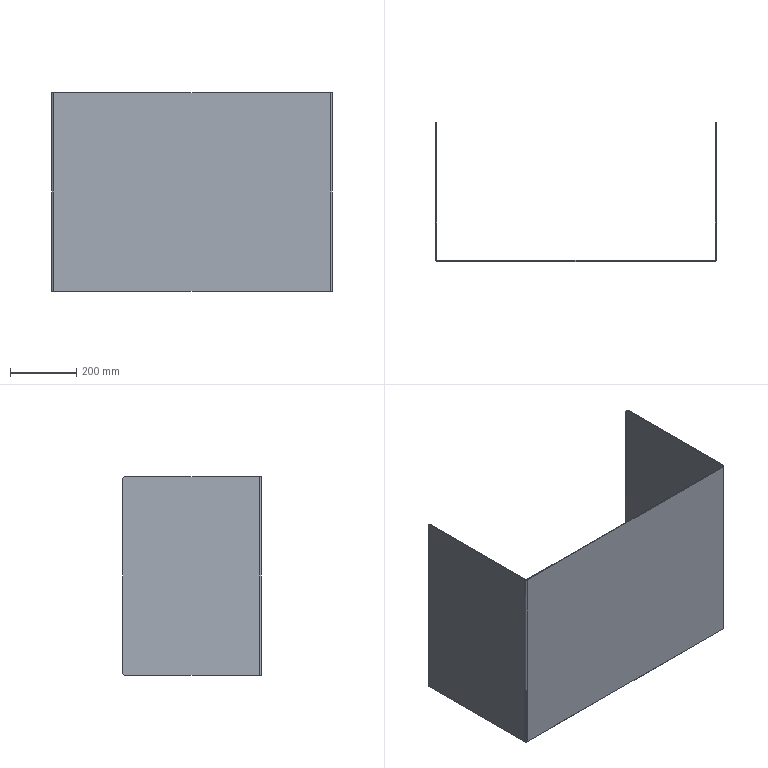Part | SolidWorks | features FlatPattern 1, ICE 1, SMBaseFlange 1, SheetMetal 1 | 1 solid | 26 faces | box 850 x 420 x 600 mm | volume 3024154 mm3 | plane 18 | cylinder 8 | commonest cylinder face diameters 12 x6 6 x2
STEP:
#1=CARTESIAN_POINT('',(850.,414.,0.));
#2=VERTEX_POINT('',#1);
#3=CARTESIAN_POINT('',(850.,420.,6.));
#4=VERTEX_POINT('',#3);
#5=CARTESIAN_POINT('',(850.,414.,6.));
#6=DIRECTION('',(1.,0.,0.));
#7=DIRECTION('',(0.,0.,1.));
#8=AXIS2_PLACEMENT_3D('',#5,#6,#7);
#9=CIRCLE('',#8,6.);
#10=EDGE_CURVE('',#2,#4,#9,.T.);
#11=ORIENTED_EDGE('',*,*,#10,.T.);
#12=CARTESIAN_POINT('',(850.,420.,594.));
#13=VERTEX_POINT('',#12);
#14=CARTESIAN_POINT('',(850.,420.,600.));
#15=DIRECTION('',(0.,0.,-1.));
#16=VECTOR('',#15,1000.);
#17=LINE('',#14,#16);
#18=EDGE_CURVE('',#13,#4,#17,.T.);
#19=ORIENTED_EDGE('',*,*,#18,.F.);
#20=CARTESIAN_POINT('',(850.,414.,600.));
#21=VERTEX_POINT('',#20);
#22=CARTESIAN_POINT('',(850.,414.,594.));
#23=DIRECTION('',(1.,0.,0.));
#24=DIRECTION('',(0.,0.,1.));
#25=AXIS2_PLACEMENT_3D('',#22,#23,#24);
#26=CIRCLE('',#25,6.);
#27=EDGE_CURVE('',#13,#21,#26,.T.);
#28=ORIENTED_EDGE('',*,*,#27,.T.);
#29=CARTESIAN_POINT('',(850.,6.,600.));
#30=VERTEX_POINT('',#29);
#31=CARTESIAN_POINT('',(850.,0.,600.));
#32=DIRECTION('',(0.,1.,0.));
#33=VECTOR('',#32,1000.);
#34=LINE('',#31,#33);
#35=EDGE_CURVE('',#30,#21,#34,.T.);
#36=ORIENTED_EDGE('',*,*,#35,.F.);
#37=CARTESIAN_POINT('',(850.,6.,0.));
#38=VERTEX_POINT('',#37);
#39=CARTESIAN_POINT('',(850.,6.,600.));
#40=DIRECTION('',(0.,0.,-1.));
#41=VECTOR('',#40,1000.);
#42=LINE('',#39,#41);
#43=EDGE_CURVE('',#30,#38,#42,.T.);
#44=ORIENTED_EDGE('',*,*,#43,.T.);
#45=CARTESIAN_POINT('',(850.,0.,0.));
#46=DIRECTION('',(0.,1.,0.));
#47=VECTOR('',#46,1000.);
#48=LINE('',#45,#47);
#49=EDGE_CURVE('',#38,#2,#48,.T.);
#50=ORIENTED_EDGE('',*,*,#49,.T.);
#51=EDGE_LOOP('',(#11,#19,#28,#36,#44,#50));
#52=FACE_OUTER_BOUND('',#51,.T.);
#53=CARTESIAN_POINT('',(850.,0.,600.));
#54=DIRECTION('',(-1.,0.,0.));
#55=DIRECTION('',(0.,0.,1.));
#56=AXIS2_PLACEMENT_3D('',#53,#54,#55);
#57=PLANE('',#56);
#58=ADVANCED_FACE('',(#52),#57,.F.);
#59=CARTESIAN_POINT('',(847.,420.,594.));
#60=VERTEX_POINT('',#59);
#61=CARTESIAN_POINT('',(847.,420.,6.));
#62=VERTEX_POINT('',#61);
#63=CARTESIAN_POINT('',(847.,420.,600.));
#64=DIRECTION('',(0.,0.,-1.));
#65=VECTOR('',#64,1000.);
#66=LINE('',#63,#65);
#67=EDGE_CURVE('',#60,#62,#66,.T.);
#68=ORIENTED_EDGE('',*,*,#67,.T.);
#69=CARTESIAN_POINT('',(847.,414.,0.));
#70=VERTEX_POINT('',#69);
#71=CARTESIAN_POINT('',(847.,414.,6.));
#72=DIRECTION('',(1.,0.,0.));
#73=DIRECTION('',(0.,0.,1.));
#74=AXIS2_PLACEMENT_3D('',#71,#72,#73);
#75=CIRCLE('',#74,6.);
#76=EDGE_CURVE('',#70,#62,#75,.T.);
#77=ORIENTED_EDGE('',*,*,#76,.F.);
#78=CARTESIAN_POINT('',(847.,6.,0.));
#79=VERTEX_POINT('',#78);
#80=CARTESIAN_POINT('',(847.,0.,0.));
#81=DIRECTION('',(0.,1.,0.));
#82=VECTOR('',#81,1000.);
#83=LINE('',#80,#82);
#84=EDGE_CURVE('',#79,#70,#83,.T.);
#85=ORIENTED_EDGE('',*,*,#84,.F.);
#86=CARTESIAN_POINT('',(847.,6.,600.));
#87=VERTEX_POINT('',#86);
#88=CARTESIAN_POINT('',(847.,6.,600.));
#89=DIRECTION('',(0.,0.,-1.));
#90=VECTOR('',#89,1000.);
#91=LINE('',#88,#90);
#92=EDGE_CURVE('',#87,#79,#91,.T.);
#93=ORIENTED_EDGE('',*,*,#92,.F.);
#94=CARTESIAN_POINT('',(847.,414.,600.));
#95=VERTEX_POINT('',#94);
#96=CARTESIAN_POINT('',(847.,0.,600.));
#97=DIRECTION('',(0.,1.,0.));
#98=VECTOR('',#97,1000.);
#99=LINE('',#96,#98);
#100=EDGE_CURVE('',#87,#95,#99,.T.);
#101=ORIENTED_EDGE('',*,*,#100,.T.);
#102=CARTESIAN_POINT('',(847.,414.,594.));
#103=DIRECTION('',(1.,0.,0.));
#104=DIRECTION('',(0.,0.,1.));
#105=AXIS2_PLACEMENT_3D('',#102,#103,#104);
#106=CIRCLE('',#105,6.);
#107=EDGE_CURVE('',#60,#95,#106,.T.);
#108=ORIENTED_EDGE('',*,*,#107,.F.);
#109=EDGE_LOOP('',(#68,#77,#85,#93,#101,#108));
#110=FACE_OUTER_BOUND('',#109,.T.);
#111=CARTESIAN_POINT('',(847.,0.,600.));
#112=DIRECTION('',(-1.,0.,0.));
#113=DIRECTION('',(0.,0.,1.));
#114=AXIS2_PLACEMENT_3D('',#111,#112,#113);
#115=PLANE('',#114);
#116=ADVANCED_FACE('',(#110),#115,.T.);
#117=ORIENTED_EDGE('',*,*,#18,.T.);
#118=CARTESIAN_POINT('',(847.,420.,6.));
#119=DIRECTION('',(1.,0.,0.));
#120=VECTOR('',#119,1000.);
#121=LINE('',#118,#120);
#122=EDGE_CURVE('',#62,#4,#121,.T.);
#123=ORIENTED_EDGE('',*,*,#122,.F.);
#124=ORIENTED_EDGE('',*,*,#67,.F.);
#125=CARTESIAN_POINT('',(847.,420.,594.));
#126=DIRECTION('',(1.,0.,0.));
#127=VECTOR('',#126,1000.);
#128=LINE('',#125,#127);
#129=EDGE_CURVE('',#60,#13,#128,.T.);
#130=ORIENTED_EDGE('',*,*,#129,.T.);
#131=EDGE_LOOP('',(#117,#123,#124,#130));
#132=FACE_OUTER_BOUND('',#131,.T.);
#133=CARTESIAN_POINT('',(847.,420.,600.));
#134=DIRECTION('',(0.,1.,0.));
#135=DIRECTION('',(0.,0.,1.));
#136=AXIS2_PLACEMENT_3D('',#133,#134,#135);
#137=PLANE('',#136);
#138=ADVANCED_FACE('',(#132),#137,.T.);
#139=CARTESIAN_POINT('',(3.,414.,0.));
#140=VERTEX_POINT('',#139);
#141=CARTESIAN_POINT('',(3.,6.,0.));
#142=VERTEX_POINT('',#141);
#143=CARTESIAN_POINT('',(3.,0.,0.));
#144=DIRECTION('',(0.,-1.,0.));
#145=VECTOR('',#144,1000.);
#146=LINE('',#143,#145);
#147=EDGE_CURVE('',#140,#142,#146,.T.);
#148=ORIENTED_EDGE('',*,*,#147,.F.);
#149=CARTESIAN_POINT('',(3.,420.,6.));
#150=VERTEX_POINT('',#149);
#151=CARTESIAN_POINT('',(3.,414.,6.));
#152=DIRECTION('',(-1.,0.,0.));
#153=DIRECTION('',(0.,0.,-1.));
#154=AXIS2_PLACEMENT_3D('',#151,#152,#153);
#155=CIRCLE('',#154,6.);
#156=EDGE_CURVE('',#150,#140,#155,.T.);
#157=ORIENTED_EDGE('',*,*,#156,.F.);
#158=CARTESIAN_POINT('',(3.,420.,594.));
#159=VERTEX_POINT('',#158);
#160=CARTESIAN_POINT('',(3.,420.,600.));
#161=DIRECTION('',(0.,0.,-1.));
#162=VECTOR('',#161,1000.);
#163=LINE('',#160,#162);
#164=EDGE_CURVE('',#159,#150,#163,.T.);
#165=ORIENTED_EDGE('',*,*,#164,.F.);
#166=CARTESIAN_POINT('',(3.,414.,600.));
#167=VERTEX_POINT('',#166);
#168=CARTESIAN_POINT('',(3.,414.,594.));
#169=DIRECTION('',(-1.,0.,0.));
#170=DIRECTION('',(0.,0.,-1.));
#171=AXIS2_PLACEMENT_3D('',#168,#169,#170);
#172=CIRCLE('',#171,6.);
#173=EDGE_CURVE('',#167,#159,#172,.T.);
#174=ORIENTED_EDGE('',*,*,#173,.F.);
#175=CARTESIAN_POINT('',(3.,6.,600.));
#176=VERTEX_POINT('',#175);
#177=CARTESIAN_POINT('',(3.,0.,600.));
#178=DIRECTION('',(0.,-1.,0.));
#179=VECTOR('',#178,1000.);
#180=LINE('',#177,#179);
#181=EDGE_CURVE('',#167,#176,#180,.T.);
#182=ORIENTED_EDGE('',*,*,#181,.T.);
#183=CARTESIAN_POINT('',(3.,6.,600.));
#184=DIRECTION('',(0.,0.,-1.));
#185=VECTOR('',#184,1000.);
#186=LINE('',#183,#185);
#187=EDGE_CURVE('',#176,#142,#186,.T.);
#188=ORIENTED_EDGE('',*,*,#187,.T.);
#189=EDGE_LOOP('',(#148,#157,#165,#174,#182,#188));
#190=FACE_OUTER_BOUND('',#189,.T.);
#191=CARTESIAN_POINT('',(3.,0.,600.));
#192=DIRECTION('',(1.,0.,0.));
#193=DIRECTION('',(0.,0.,-1.));
#194=AXIS2_PLACEMENT_3D('',#191,#192,#193);
#195=PLANE('',#194);
#196=ADVANCED_FACE('',(#190),#195,.T.);
#197=CARTESIAN_POINT('',(0.,420.,6.));
#198=VERTEX_POINT('',#197);
#199=CARTESIAN_POINT('',(0.,414.,0.));
#200=VERTEX_POINT('',#199);
#201=CARTESIAN_POINT('',(0.,414.,6.));
#202=DIRECTION('',(-1.,0.,0.));
#203=DIRECTION('',(0.,0.,-1.));
#204=AXIS2_PLACEMENT_3D('',#201,#202,#203);
#205=CIRCLE('',#204,6.);
#206=EDGE_CURVE('',#198,#200,#205,.T.);
#207=ORIENTED_EDGE('',*,*,#206,.T.);
#208=CARTESIAN_POINT('',(0.,6.,0.));
#209=VERTEX_POINT('',#208);
#210=CARTESIAN_POINT('',(0.,0.,0.));
#211=DIRECTION('',(0.,-1.,0.));
#212=VECTOR('',#211,1000.);
#213=LINE('',#210,#212);
#214=EDGE_CURVE('',#200,#209,#213,.T.);
#215=ORIENTED_EDGE('',*,*,#214,.T.);
#216=CARTESIAN_POINT('',(0.,6.,600.));
#217=VERTEX_POINT('',#216);
#218=CARTESIAN_POINT('',(0.,6.,600.));
#219=DIRECTION('',(0.,0.,-1.));
#220=VECTOR('',#219,1000.);
#221=LINE('',#218,#220);
#222=EDGE_CURVE('',#217,#209,#221,.T.);
#223=ORIENTED_EDGE('',*,*,#222,.F.);
#224=CARTESIAN_POINT('',(0.,414.,600.));
#225=VERTEX_POINT('',#224);
#226=CARTESIAN_POINT('',(0.,0.,600.));
#227=DIRECTION('',(0.,-1.,0.));
#228=VECTOR('',#227,1000.);
#229=LINE('',#226,#228);
#230=EDGE_CURVE('',#225,#217,#229,.T.);
#231=ORIENTED_EDGE('',*,*,#230,.F.);
#232=CARTESIAN_POINT('',(0.,420.,594.));
#233=VERTEX_POINT('',#232);
#234=CARTESIAN_POINT('',(0.,414.,594.));
#235=DIRECTION('',(-1.,0.,0.));
#236=DIRECTION('',(0.,0.,-1.));
#237=AXIS2_PLACEMENT_3D('',#234,#235,#236);
#238=CIRCLE('',#237,6.);
#239=EDGE_CURVE('',#225,#233,#238,.T.);
#240=ORIENTED_EDGE('',*,*,#239,.T.);
#241=CARTESIAN_POINT('',(0.,420.,600.));
#242=DIRECTION('',(0.,0.,-1.));
#243=VECTOR('',#242,1000.);
#244=LINE('',#241,#243);
#245=EDGE_CURVE('',#233,#198,#244,.T.);
#246=ORIENTED_EDGE('',*,*,#245,.T.);
#247=EDGE_LOOP('',(#207,#215,#223,#231,#240,#246));
#248=FACE_OUTER_BOUND('',#247,.T.);
#249=CARTESIAN_POINT('',(0.,0.,600.));
#250=DIRECTION('',(1.,0.,0.));
#251=DIRECTION('',(0.,0.,-1.));
#252=AXIS2_PLACEMENT_3D('',#249,#250,#251);
#253=PLANE('',#252);
#254=ADVANCED_FACE('',(#248),#253,.F.);
#255=ORIENTED_EDGE('',*,*,#35,.T.);
#256=CARTESIAN_POINT('',(847.,414.,600.));
#257=DIRECTION('',(1.,0.,0.));
#258=VECTOR('',#257,1000.);
#259=LINE('',#256,#258);
#260=EDGE_CURVE('',#95,#21,#259,.T.);
#261=ORIENTED_EDGE('',*,*,#260,.F.);
#262=ORIENTED_EDGE('',*,*,#100,.F.);
#263=CARTESIAN_POINT('',(847.,6.,600.));
#264=DIRECTION('',(1.,0.,0.));
#265=VECTOR('',#264,1000.);
#266=LINE('',#263,#265);
#267=EDGE_CURVE('',#87,#30,#266,.T.);
#268=ORIENTED_EDGE('',*,*,#267,.T.);
#269=EDGE_LOOP('',(#255,#261,#262,#268));
#270=FACE_OUTER_BOUND('',#269,.T.);
#271=CARTESIAN_POINT('',(844.,6.,600.));
#272=DIRECTION('',(0.,0.,1.));
#273=DIRECTION('',(1.,0.,0.));
#274=AXIS2_PLACEMENT_3D('',#271,#272,#273);
#275=PLANE('',#274);
#276=ADVANCED_FACE('',(#270),#275,.T.);
#277=CARTESIAN_POINT('',(3.,420.,6.));
#278=DIRECTION('',(-1.,0.,0.));
#279=VECTOR('',#278,1000.);
#280=LINE('',#277,#279);
#281=EDGE_CURVE('',#150,#198,#280,.T.);
#282=ORIENTED_EDGE('',*,*,#281,.T.);
#283=ORIENTED_EDGE('',*,*,#245,.F.);
#284=CARTESIAN_POINT('',(3.,420.,594.));
#285=DIRECTION('',(-1.,0.,0.));
#286=VECTOR('',#285,1000.);
#287=LINE('',#284,#286);
#288=EDGE_CURVE('',#159,#233,#287,.T.);
#289=ORIENTED_EDGE('',*,*,#288,.F.);
#290=ORIENTED_EDGE('',*,*,#164,.T.);
#291=EDGE_LOOP('',(#282,#283,#289,#290));
#292=FACE_OUTER_BOUND('',#291,.T.);
#293=CARTESIAN_POINT('',(0.,420.,600.));
#294=DIRECTION('',(0.,1.,0.));
#295=DIRECTION('',(0.,0.,1.));
#296=AXIS2_PLACEMENT_3D('',#293,#294,#295);
#297=PLANE('',#296);
#298=ADVANCED_FACE('',(#292),#297,.T.);
#299=CARTESIAN_POINT('',(0.,6.,600.));
#300=DIRECTION('',(1.,0.,0.));
#301=VECTOR('',#300,1000.);
#302=LINE('',#299,#301);
#303=EDGE_CURVE('',#217,#176,#302,.T.);
#304=ORIENTED_EDGE('',*,*,#303,.F.);
#305=CARTESIAN_POINT('',(6.,0.,600.));
#306=VERTEX_POINT('',#305);
#307=CARTESIAN_POINT('',(6.,6.,600.));
#308=DIRECTION('',(0.,0.,1.));
#309=DIRECTION('',(-1.,0.,0.));
#310=AXIS2_PLACEMENT_3D('',#307,#308,#309);
#311=CIRCLE('',#310,6.);
#312=EDGE_CURVE('',#217,#306,#311,.T.);
#313=ORIENTED_EDGE('',*,*,#312,.T.);
#314=CARTESIAN_POINT('',(6.,3.,600.));
#315=VERTEX_POINT('',#314);
#316=CARTESIAN_POINT('',(6.,3.,600.));
#317=DIRECTION('',(0.,-1.,0.));
#318=VECTOR('',#317,1000.);
#319=LINE('',#316,#318);
#320=EDGE_CURVE('',#315,#306,#319,.T.);
#321=ORIENTED_EDGE('',*,*,#320,.F.);
#322=CARTESIAN_POINT('',(6.,6.,600.));
#323=DIRECTION('',(0.,0.,1.));
#324=DIRECTION('',(1.,0.,0.));
#325=AXIS2_PLACEMENT_3D('',#322,#323,#324);
#326=CIRCLE('',#325,3.);
#327=EDGE_CURVE('',#176,#315,#326,.T.);
#328=ORIENTED_EDGE('',*,*,#327,.F.);
#329=EDGE_LOOP('',(#304,#313,#321,#328));
#330=FACE_OUTER_BOUND('',#329,.T.);
#331=CARTESIAN_POINT('',(0.,6.,600.));
#332=DIRECTION('',(0.,0.,1.));
#333=DIRECTION('',(1.,0.,0.));
#334=AXIS2_PLACEMENT_3D('',#331,#332,#333);
#335=PLANE('',#334);
#336=ADVANCED_FACE('',(#330),#335,.T.);
#337=CARTESIAN_POINT('',(3.,414.,600.));
#338=DIRECTION('',(-1.,0.,0.));
#339=VECTOR('',#338,1000.);
#340=LINE('',#337,#339);
#341=EDGE_CURVE('',#167,#225,#340,.T.);
#342=ORIENTED_EDGE('',*,*,#341,.T.);
#343=ORIENTED_EDGE('',*,*,#230,.T.);
#344=ORIENTED_EDGE('',*,*,#303,.T.);
#345=ORIENTED_EDGE('',*,*,#181,.F.);
#346=EDGE_LOOP('',(#342,#343,#344,#345));
#347=FACE_OUTER_BOUND('',#346,.T.);
#348=CARTESIAN_POINT('',(6.,3.,600.));
#349=DIRECTION('',(0.,0.,1.));
#350=DIRECTION('',(1.,0.,0.));
#351=AXIS2_PLACEMENT_3D('',#348,#349,#350);
#352=PLANE('',#351);
#353=ADVANCED_FACE('',(#347),#352,.T.);
#354=CARTESIAN_POINT('',(6.,0.,0.));
#355=VERTEX_POINT('',#354);
#356=CARTESIAN_POINT('',(6.,3.,0.));
#357=VERTEX_POINT('',#356);
#358=CARTESIAN_POINT('',(6.,0.,0.));
#359=DIRECTION('',(0.,1.,0.));
#360=VECTOR('',#359,1000.);
#361=LINE('',#358,#360);
#362=EDGE_CURVE('',#355,#357,#361,.T.);
#363=ORIENTED_EDGE('',*,*,#362,.F.);
#364=CARTESIAN_POINT('',(6.,6.,0.));
#365=DIRECTION('',(0.,0.,1.));
#366=DIRECTION('',(-1.,0.,0.));
#367=AXIS2_PLACEMENT_3D('',#364,#365,#366);
#368=CIRCLE('',#367,6.);
#369=EDGE_CURVE('',#209,#355,#368,.T.);
#370=ORIENTED_EDGE('',*,*,#369,.F.);
#371=CARTESIAN_POINT('',(3.,6.,0.));
#372=DIRECTION('',(-1.,0.,0.));
#373=VECTOR('',#372,1000.);
#374=LINE('',#371,#373);
#375=EDGE_CURVE('',#142,#209,#374,.T.);
#376=ORIENTED_EDGE('',*,*,#375,.F.);
#377=CARTESIAN_POINT('',(6.,6.,0.));
#378=DIRECTION('',(0.,0.,1.));
#379=DIRECTION('',(1.,0.,0.));
#380=AXIS2_PLACEMENT_3D('',#377,#378,#379);
#381=CIRCLE('',#380,3.);
#382=EDGE_CURVE('',#142,#357,#381,.T.);
#383=ORIENTED_EDGE('',*,*,#382,.T.);
#384=EDGE_LOOP('',(#363,#370,#376,#383));
#385=FACE_OUTER_BOUND('',#384,.T.);
#386=CARTESIAN_POINT('',(6.,0.,0.));
#387=DIRECTION('',(0.,0.,-1.));
#388=DIRECTION('',(-1.,0.,0.));
#389=AXIS2_PLACEMENT_3D('',#386,#387,#388);
#390=PLANE('',#389);
#391=ADVANCED_FACE('',(#385),#390,.T.);
#392=CARTESIAN_POINT('',(844.,0.,0.));
#393=VERTEX_POINT('',#392);
#394=CARTESIAN_POINT('',(0.,0.,0.));
#395=DIRECTION('',(1.,0.,0.));
#396=VECTOR('',#395,1000.);
#397=LINE('',#394,#396);
#398=EDGE_CURVE('',#355,#393,#397,.T.);
#399=ORIENTED_EDGE('',*,*,#398,.F.);
#400=ORIENTED_EDGE('',*,*,#362,.T.);
#401=CARTESIAN_POINT('',(844.,3.,0.));
#402=VERTEX_POINT('',#401);
#403=CARTESIAN_POINT('',(0.,3.,0.));
#404=DIRECTION('',(1.,0.,0.));
#405=VECTOR('',#404,1000.);
#406=LINE('',#403,#405);
#407=EDGE_CURVE('',#357,#402,#406,.T.);
#408=ORIENTED_EDGE('',*,*,#407,.T.);
#409=CARTESIAN_POINT('',(844.,3.,0.));
#410=DIRECTION('',(0.,-1.,0.));
#411=VECTOR('',#410,1000.);
#412=LINE('',#409,#411);
#413=EDGE_CURVE('',#402,#393,#412,.T.);
#414=ORIENTED_EDGE('',*,*,#413,.T.);
#415=EDGE_LOOP('',(#399,#400,#408,#414));
#416=FACE_OUTER_BOUND('',#415,.T.);
#417=CARTESIAN_POINT('',(3.,6.,0.));
#418=DIRECTION('',(0.,0.,-1.));
#419=DIRECTION('',(-1.,0.,0.));
#420=AXIS2_PLACEMENT_3D('',#417,#418,#419);
#421=PLANE('',#420);
#422=ADVANCED_FACE('',(#416),#421,.T.);
#423=CARTESIAN_POINT('',(844.,0.,600.));
#424=VERTEX_POINT('',#423);
#425=CARTESIAN_POINT('',(844.,3.,600.));
#426=VERTEX_POINT('',#425);
#427=CARTESIAN_POINT('',(844.,0.,600.));
#428=DIRECTION('',(0.,1.,0.));
#429=VECTOR('',#428,1000.);
#430=LINE('',#427,#429);
#431=EDGE_CURVE('',#424,#426,#430,.T.);
#432=ORIENTED_EDGE('',*,*,#431,.F.);
#433=CARTESIAN_POINT('',(844.,6.,600.));
#434=DIRECTION('',(0.,0.,1.));
#435=DIRECTION('',(-1.,0.,0.));
#436=AXIS2_PLACEMENT_3D('',#433,#434,#435);
#437=CIRCLE('',#436,6.);
#438=EDGE_CURVE('',#424,#30,#437,.T.);
#439=ORIENTED_EDGE('',*,*,#438,.T.);
#440=ORIENTED_EDGE('',*,*,#267,.F.);
#441=CARTESIAN_POINT('',(844.,6.,600.));
#442=DIRECTION('',(0.,0.,1.));
#443=DIRECTION('',(1.,0.,0.));
#444=AXIS2_PLACEMENT_3D('',#441,#442,#443);
#445=CIRCLE('',#444,3.);
#446=EDGE_CURVE('',#426,#87,#445,.T.);
#447=ORIENTED_EDGE('',*,*,#446,.F.);
#448=EDGE_LOOP('',(#432,#439,#440,#447));
#449=FACE_OUTER_BOUND('',#448,.T.);
#450=CARTESIAN_POINT('',(844.,0.,600.));
#451=DIRECTION('',(0.,0.,1.));
#452=DIRECTION('',(1.,0.,0.));
#453=AXIS2_PLACEMENT_3D('',#450,#451,#452);
#454=PLANE('',#453);
#455=ADVANCED_FACE('',(#449),#454,.T.);
#456=CARTESIAN_POINT('',(0.,0.,600.));
#457=DIRECTION('',(1.,0.,0.));
#458=VECTOR('',#457,1000.);
#459=LINE('',#456,#458);
#460=EDGE_CURVE('',#306,#424,#459,.T.);
#461=ORIENTED_EDGE('',*,*,#460,.T.);
#462=ORIENTED_EDGE('',*,*,#431,.T.);
#463=CARTESIAN_POINT('',(0.,3.,600.));
#464=DIRECTION('',(1.,0.,0.));
#465=VECTOR('',#464,1000.);
#466=LINE('',#463,#465);
#467=EDGE_CURVE('',#315,#426,#466,.T.);
#468=ORIENTED_EDGE('',*,*,#467,.F.);
#469=ORIENTED_EDGE('',*,*,#320,.T.);
#470=EDGE_LOOP('',(#461,#462,#468,#469));
#471=FACE_OUTER_BOUND('',#470,.T.);
#472=CARTESIAN_POINT('',(847.,6.,600.));
#473=DIRECTION('',(0.,0.,1.));
#474=DIRECTION('',(1.,0.,0.));
#475=AXIS2_PLACEMENT_3D('',#472,#473,#474);
#476=PLANE('',#475);
#477=ADVANCED_FACE('',(#471),#476,.T.);
#478=CARTESIAN_POINT('',(850.,6.,0.));
#479=DIRECTION('',(-1.,0.,0.));
#480=VECTOR('',#479,1000.);
#481=LINE('',#478,#480);
#482=EDGE_CURVE('',#38,#79,#481,.T.);
#483=ORIENTED_EDGE('',*,*,#482,.F.);
#484=CARTESIAN_POINT('',(844.,6.,0.));
#485=DIRECTION('',(0.,0.,1.));
#486=DIRECTION('',(-1.,0.,0.));
#487=AXIS2_PLACEMENT_3D('',#484,#485,#486);
#488=CIRCLE('',#487,6.);
#489=EDGE_CURVE('',#393,#38,#488,.T.);
#490=ORIENTED_EDGE('',*,*,#489,.F.);
#491=ORIENTED_EDGE('',*,*,#413,.F.);
#492=CARTESIAN_POINT('',(844.,6.,0.));
#493=DIRECTION('',(0.,0.,1.));
#494=DIRECTION('',(1.,0.,0.));
#495=AXIS2_PLACEMENT_3D('',#492,#493,#494);
#496=CIRCLE('',#495,3.);
#497=EDGE_CURVE('',#402,#79,#496,.T.);
#498=ORIENTED_EDGE('',*,*,#497,.T.);
#499=EDGE_LOOP('',(#483,#490,#491,#498));
#500=FACE_OUTER_BOUND('',#499,.T.);
#501=CARTESIAN_POINT('',(850.,6.,0.));
#502=DIRECTION('',(0.,0.,-1.));
#503=DIRECTION('',(-1.,0.,0.));
#504=AXIS2_PLACEMENT_3D('',#501,#502,#503);
#505=PLANE('',#504);
#506=ADVANCED_FACE('',(#500),#505,.T.);
#507=CARTESIAN_POINT('',(847.,414.,0.));
#508=DIRECTION('',(1.,0.,0.));
#509=VECTOR('',#508,1000.);
#510=LINE('',#507,#509);
#511=EDGE_CURVE('',#70,#2,#510,.T.);
#512=ORIENTED_EDGE('',*,*,#511,.T.);
#513=ORIENTED_EDGE('',*,*,#49,.F.);
#514=ORIENTED_EDGE('',*,*,#482,.T.);
#515=ORIENTED_EDGE('',*,*,#84,.T.);
#516=EDGE_LOOP('',(#512,#513,#514,#515));
#517=FACE_OUTER_BOUND('',#516,.T.);
#518=CARTESIAN_POINT('',(844.,3.,0.));
#519=DIRECTION('',(0.,0.,-1.));
#520=DIRECTION('',(-1.,0.,0.));
#521=AXIS2_PLACEMENT_3D('',#518,#519,#520);
#522=PLANE('',#521);
#523=ADVANCED_FACE('',(#517),#522,.T.);
#524=ORIENTED_EDGE('',*,*,#497,.F.);
#525=CARTESIAN_POINT('',(844.,3.,600.));
#526=DIRECTION('',(0.,0.,-1.));
#527=VECTOR('',#526,1000.);
#528=LINE('',#525,#527);
#529=EDGE_CURVE('',#426,#402,#528,.T.);
#530=ORIENTED_EDGE('',*,*,#529,.F.);
#531=ORIENTED_EDGE('',*,*,#446,.T.);
#532=ORIENTED_EDGE('',*,*,#92,.T.);
#533=EDGE_LOOP('',(#524,#530,#531,#532));
#534=FACE_OUTER_BOUND('',#533,.T.);
#535=CARTESIAN_POINT('',(844.,6.,600.));
#536=DIRECTION('',(0.,0.,-1.));
#537=DIRECTION('',(-1.,0.,0.));
#538=AXIS2_PLACEMENT_3D('',#535,#536,#537);
#539=CYLINDRICAL_SURFACE('',#538,3.);
#540=ADVANCED_FACE('',(#534),#539,.F.);
#541=ORIENTED_EDGE('',*,*,#407,.F.);
#542=CARTESIAN_POINT('',(6.,3.,600.));
#543=DIRECTION('',(0.,0.,-1.));
#544=VECTOR('',#543,1000.);
#545=LINE('',#542,#544);
#546=EDGE_CURVE('',#315,#357,#545,.T.);
#547=ORIENTED_EDGE('',*,*,#546,.F.);
#548=ORIENTED_EDGE('',*,*,#467,.T.);
#549=ORIENTED_EDGE('',*,*,#529,.T.);
#550=EDGE_LOOP('',(#541,#547,#548,#549));
#551=FACE_OUTER_BOUND('',#550,.T.);
#552=CARTESIAN_POINT('',(0.,3.,600.));
#553=DIRECTION('',(0.,1.,0.));
#554=DIRECTION('',(0.,0.,1.));
#555=AXIS2_PLACEMENT_3D('',#552,#553,#554);
#556=PLANE('',#555);
#557=ADVANCED_FACE('',(#551),#556,.T.);
#558=ORIENTED_EDGE('',*,*,#382,.F.);
#559=ORIENTED_EDGE('',*,*,#187,.F.);
#560=ORIENTED_EDGE('',*,*,#327,.T.);
#561=ORIENTED_EDGE('',*,*,#546,.T.);
#562=EDGE_LOOP('',(#558,#559,#560,#561));
#563=FACE_OUTER_BOUND('',#562,.T.);
#564=CARTESIAN_POINT('',(6.,6.,600.));
#565=DIRECTION('',(0.,0.,-1.));
#566=DIRECTION('',(-1.,0.,0.));
#567=AXIS2_PLACEMENT_3D('',#564,#565,#566);
#568=CYLINDRICAL_SURFACE('',#567,3.);
#569=ADVANCED_FACE('',(#563),#568,.F.);
#570=ORIENTED_EDGE('',*,*,#369,.T.);
#571=CARTESIAN_POINT('',(6.,0.,600.));
#572=DIRECTION('',(0.,0.,-1.));
#573=VECTOR('',#572,1000.);
#574=LINE('',#571,#573);
#575=EDGE_CURVE('',#306,#355,#574,.T.);
#576=ORIENTED_EDGE('',*,*,#575,.F.);
#577=ORIENTED_EDGE('',*,*,#312,.F.);
#578=ORIENTED_EDGE('',*,*,#222,.T.);
#579=EDGE_LOOP('',(#570,#576,#577,#578));
#580=FACE_OUTER_BOUND('',#579,.T.);
#581=CARTESIAN_POINT('',(6.,6.,600.));
#582=DIRECTION('',(0.,0.,-1.));
#583=DIRECTION('',(-1.,0.,0.));
#584=AXIS2_PLACEMENT_3D('',#581,#582,#583);
#585=CYLINDRICAL_SURFACE('',#584,6.);
#586=ADVANCED_FACE('',(#580),#585,.T.);
#587=ORIENTED_EDGE('',*,*,#398,.T.);
#588=CARTESIAN_POINT('',(844.,0.,600.));
#589=DIRECTION('',(0.,0.,-1.));
#590=VECTOR('',#589,1000.);
#591=LINE('',#588,#590);
#592=EDGE_CURVE('',#424,#393,#591,.T.);
#593=ORIENTED_EDGE('',*,*,#592,.F.);
#594=ORIENTED_EDGE('',*,*,#460,.F.);
#595=ORIENTED_EDGE('',*,*,#575,.T.);
#596=EDGE_LOOP('',(#587,#593,#594,#595));
#597=FACE_OUTER_BOUND('',#596,.T.);
#598=CARTESIAN_POINT('',(0.,0.,600.));
#599=DIRECTION('',(0.,1.,0.));
#600=DIRECTION('',(0.,0.,1.));
#601=AXIS2_PLACEMENT_3D('',#598,#599,#600);
#602=PLANE('',#601);
#603=ADVANCED_FACE('',(#597),#602,.F.);
#604=ORIENTED_EDGE('',*,*,#489,.T.);
#605=ORIENTED_EDGE('',*,*,#43,.F.);
#606=ORIENTED_EDGE('',*,*,#438,.F.);
#607=ORIENTED_EDGE('',*,*,#592,.T.);
#608=EDGE_LOOP('',(#604,#605,#606,#607));
#609=FACE_OUTER_BOUND('',#608,.T.);
#610=CARTESIAN_POINT('',(844.,6.,600.));
#611=DIRECTION('',(0.,0.,-1.));
#612=DIRECTION('',(-1.,0.,0.));
#613=AXIS2_PLACEMENT_3D('',#610,#611,#612);
#614=CYLINDRICAL_SURFACE('',#613,6.);
#615=ADVANCED_FACE('',(#609),#614,.T.);
#616=ORIENTED_EDGE('',*,*,#214,.F.);
#617=CARTESIAN_POINT('',(3.,414.,0.));
#618=DIRECTION('',(-1.,0.,0.));
#619=VECTOR('',#618,1000.);
#620=LINE('',#617,#619);
#621=EDGE_CURVE('',#140,#200,#620,.T.);
#622=ORIENTED_EDGE('',*,*,#621,.F.);
#623=ORIENTED_EDGE('',*,*,#147,.T.);
#624=ORIENTED_EDGE('',*,*,#375,.T.);
#625=EDGE_LOOP('',(#616,#622,#623,#624));
#626=FACE_OUTER_BOUND('',#625,.T.);
#627=CARTESIAN_POINT('',(844.,6.,0.));
#628=DIRECTION('',(0.,0.,1.));
#629=DIRECTION('',(1.,0.,0.));
#630=AXIS2_PLACEMENT_3D('',#627,#628,#629);
#631=PLANE('',#630);
#632=ADVANCED_FACE('',(#626),#631,.F.);
#633=ORIENTED_EDGE('',*,*,#173,.T.);
#634=ORIENTED_EDGE('',*,*,#288,.T.);
#635=ORIENTED_EDGE('',*,*,#239,.F.);
#636=ORIENTED_EDGE('',*,*,#341,.F.);
#637=EDGE_LOOP('',(#633,#634,#635,#636));
#638=FACE_OUTER_BOUND('',#637,.T.);
#639=CARTESIAN_POINT('',(3.,414.,594.));
#640=DIRECTION('',(1.,0.,0.));
#641=DIRECTION('',(0.,0.,-1.));
#642=AXIS2_PLACEMENT_3D('',#639,#640,#641);
#643=CYLINDRICAL_SURFACE('',#642,6.);
#644=ADVANCED_FACE('',(#638),#643,.T.);
#645=ORIENTED_EDGE('',*,*,#107,.T.);
#646=ORIENTED_EDGE('',*,*,#260,.T.);
#647=ORIENTED_EDGE('',*,*,#27,.F.);
#648=ORIENTED_EDGE('',*,*,#129,.F.);
#649=EDGE_LOOP('',(#645,#646,#647,#648));
#650=FACE_OUTER_BOUND('',#649,.T.);
#651=CARTESIAN_POINT('',(847.,414.,594.));
#652=DIRECTION('',(-1.,0.,0.));
#653=DIRECTION('',(0.,0.,1.));
#654=AXIS2_PLACEMENT_3D('',#651,#652,#653);
#655=CYLINDRICAL_SURFACE('',#654,6.);
#656=ADVANCED_FACE('',(#650),#655,.T.);
#657=ORIENTED_EDGE('',*,*,#156,.T.);
#658=ORIENTED_EDGE('',*,*,#621,.T.);
#659=ORIENTED_EDGE('',*,*,#206,.F.);
#660=ORIENTED_EDGE('',*,*,#281,.F.);
#661=EDGE_LOOP('',(#657,#658,#659,#660));
#662=FACE_OUTER_BOUND('',#661,.T.);
#663=CARTESIAN_POINT('',(3.,414.,6.));
#664=DIRECTION('',(1.,0.,0.));
#665=DIRECTION('',(0.,0.,-1.));
#666=AXIS2_PLACEMENT_3D('',#663,#664,#665);
#667=CYLINDRICAL_SURFACE('',#666,6.);
#668=ADVANCED_FACE('',(#662),#667,.T.);
#669=ORIENTED_EDGE('',*,*,#76,.T.);
#670=ORIENTED_EDGE('',*,*,#122,.T.);
#671=ORIENTED_EDGE('',*,*,#10,.F.);
#672=ORIENTED_EDGE('',*,*,#511,.F.);
#673=EDGE_LOOP('',(#669,#670,#671,#672));
#674=FACE_OUTER_BOUND('',#673,.T.);
#675=CARTESIAN_POINT('',(847.,414.,6.));
#676=DIRECTION('',(-1.,0.,0.));
#677=DIRECTION('',(0.,0.,1.));
#678=AXIS2_PLACEMENT_3D('',#675,#676,#677);
#679=CYLINDRICAL_SURFACE('',#678,6.);
#680=ADVANCED_FACE('',(#674),#679,.T.);
#681=CLOSED_SHELL('',(#58,#116,#138,#196,#254,#276,#298,#336,#353,#391,#422,#455,#477,#506,#523,#540,#557,#569,#586,#603,#615,#632,#644,#656,#668,#680));
#682=MANIFOLD_SOLID_BREP('',#681);
#683=CARTESIAN_POINT('',(0.,0.,0.));
#684=DIRECTION('',(0.,0.,1.));
#685=DIRECTION('',(1.,0.,0.));
#686=AXIS2_PLACEMENT_3D('',#683,#684,#685);
#687=(LENGTH_UNIT()NAMED_UNIT(*)SI_UNIT(.MILLI.,.METRE.));
#688=UNCERTAINTY_MEASURE_WITH_UNIT(LENGTH_MEASURE(0.00001),#687,'','');
#689=(NAMED_UNIT(*)PLANE_ANGLE_UNIT()SI_UNIT($,.RADIAN.));
#690=(NAMED_UNIT(*)SI_UNIT($,.STERADIAN.)SOLID_ANGLE_UNIT());
#691=(GEOMETRIC_REPRESENTATION_CONTEXT(3)GLOBAL_UNCERTAINTY_ASSIGNED_CONTEXT((#688))GLOBAL_UNIT_ASSIGNED_CONTEXT((#687,#689,#690))REPRESENTATION_CONTEXT('',''));
#692=ADVANCED_BREP_SHAPE_REPRESENTATION('',(#682,#686),#691);